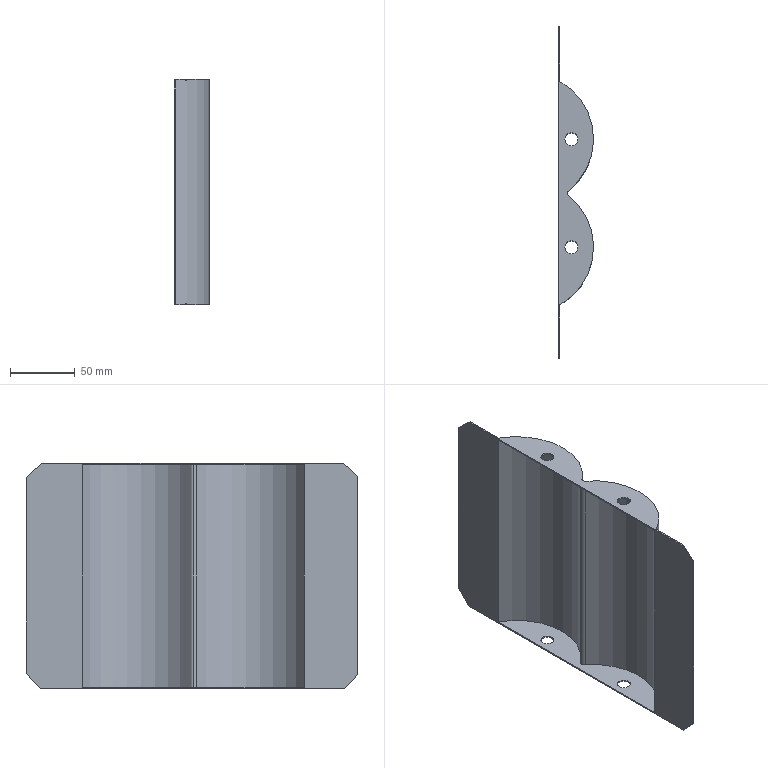Part | SolidWorks | features Chamfer 2, Extrusion 1, ICE 1, Shell 1 | 1 solid | 29 faces | box 27.127 x 256 x 174 mm | volume 56067 mm3 | cylinder 16 | plane 13 | commonest cylinder face diameters 10 x8 4 x2 6 x2 100 x2 102 x2
STEP:
#1=CARTESIAN_POINT('',(5.,168.7,173.));
#2=VERTEX_POINT('',#1);
#3=CARTESIAN_POINT('',(15.,168.7,173.));
#4=VERTEX_POINT('',#3);
#5=CARTESIAN_POINT('',(10.,168.7,173.));
#6=DIRECTION('',(0.,0.,1.));
#7=DIRECTION('',(1.,0.,0.));
#8=AXIS2_PLACEMENT_3D('',#5,#6,#7);
#9=CIRCLE('',#8,5.);
#10=EDGE_CURVE('',#2,#4,#9,.T.);
#11=ORIENTED_EDGE('',*,*,#10,.F.);
#12=CARTESIAN_POINT('',(5.,168.7,174.));
#13=VERTEX_POINT('',#12);
#14=CARTESIAN_POINT('',(5.,168.7,-28.));
#15=DIRECTION('',(0.,0.,1.));
#16=VECTOR('',#15,1000.);
#17=LINE('',#14,#16);
#18=EDGE_CURVE('',#2,#13,#17,.T.);
#19=ORIENTED_EDGE('',*,*,#18,.T.);
#20=CARTESIAN_POINT('',(15.,168.7,174.));
#21=VERTEX_POINT('',#20);
#22=CARTESIAN_POINT('',(10.,168.7,174.));
#23=DIRECTION('',(0.,0.,1.));
#24=DIRECTION('',(1.,0.,0.));
#25=AXIS2_PLACEMENT_3D('',#22,#23,#24);
#26=CIRCLE('',#25,5.);
#27=EDGE_CURVE('',#13,#21,#26,.T.);
#28=ORIENTED_EDGE('',*,*,#27,.T.);
#29=CARTESIAN_POINT('',(15.,168.7,-28.));
#30=DIRECTION('',(0.,0.,1.));
#31=VECTOR('',#30,1000.);
#32=LINE('',#29,#31);
#33=EDGE_CURVE('',#4,#21,#32,.T.);
#34=ORIENTED_EDGE('',*,*,#33,.F.);
#35=EDGE_LOOP('',(#11,#19,#28,#34));
#36=FACE_OUTER_BOUND('',#35,.T.);
#37=CARTESIAN_POINT('',(10.,168.7,-28.));
#38=DIRECTION('',(0.,0.,1.));
#39=DIRECTION('',(1.,0.,0.));
#40=AXIS2_PLACEMENT_3D('',#37,#38,#39);
#41=CYLINDRICAL_SURFACE('',#40,5.);
#42=ADVANCED_FACE('',(#36),#41,.F.);
#43=CARTESIAN_POINT('',(5.,85.3,173.));
#44=VERTEX_POINT('',#43);
#45=CARTESIAN_POINT('',(15.,85.3,173.));
#46=VERTEX_POINT('',#45);
#47=CARTESIAN_POINT('',(10.,85.3,173.));
#48=DIRECTION('',(0.,0.,1.));
#49=DIRECTION('',(1.,0.,0.));
#50=AXIS2_PLACEMENT_3D('',#47,#48,#49);
#51=CIRCLE('',#50,5.);
#52=EDGE_CURVE('',#44,#46,#51,.T.);
#53=ORIENTED_EDGE('',*,*,#52,.F.);
#54=CARTESIAN_POINT('',(5.,85.3,174.));
#55=VERTEX_POINT('',#54);
#56=CARTESIAN_POINT('',(5.,85.3,-28.));
#57=DIRECTION('',(0.,0.,1.));
#58=VECTOR('',#57,1000.);
#59=LINE('',#56,#58);
#60=EDGE_CURVE('',#44,#55,#59,.T.);
#61=ORIENTED_EDGE('',*,*,#60,.T.);
#62=CARTESIAN_POINT('',(15.,85.3,174.));
#63=VERTEX_POINT('',#62);
#64=CARTESIAN_POINT('',(10.,85.3,174.));
#65=DIRECTION('',(0.,0.,1.));
#66=DIRECTION('',(1.,0.,0.));
#67=AXIS2_PLACEMENT_3D('',#64,#65,#66);
#68=CIRCLE('',#67,5.);
#69=EDGE_CURVE('',#55,#63,#68,.T.);
#70=ORIENTED_EDGE('',*,*,#69,.T.);
#71=CARTESIAN_POINT('',(15.,85.3,-28.));
#72=DIRECTION('',(0.,0.,1.));
#73=VECTOR('',#72,1000.);
#74=LINE('',#71,#73);
#75=EDGE_CURVE('',#46,#63,#74,.T.);
#76=ORIENTED_EDGE('',*,*,#75,.F.);
#77=EDGE_LOOP('',(#53,#61,#70,#76));
#78=FACE_OUTER_BOUND('',#77,.T.);
#79=CARTESIAN_POINT('',(10.,85.3,-28.));
#80=DIRECTION('',(0.,0.,1.));
#81=DIRECTION('',(1.,0.,0.));
#82=AXIS2_PLACEMENT_3D('',#79,#80,#81);
#83=CYLINDRICAL_SURFACE('',#82,5.);
#84=ADVANCED_FACE('',(#78),#83,.F.);
#85=CARTESIAN_POINT('',(5.,168.7,0.));
#86=VERTEX_POINT('',#85);
#87=CARTESIAN_POINT('',(15.,168.7,0.));
#88=VERTEX_POINT('',#87);
#89=CARTESIAN_POINT('',(10.,168.7,0.));
#90=DIRECTION('',(0.,0.,1.));
#91=DIRECTION('',(1.,0.,0.));
#92=AXIS2_PLACEMENT_3D('',#89,#90,#91);
#93=CIRCLE('',#92,5.);
#94=EDGE_CURVE('',#86,#88,#93,.T.);
#95=ORIENTED_EDGE('',*,*,#94,.F.);
#96=CARTESIAN_POINT('',(5.,168.7,1.));
#97=VERTEX_POINT('',#96);
#98=CARTESIAN_POINT('',(5.,168.7,-28.));
#99=DIRECTION('',(0.,0.,1.));
#100=VECTOR('',#99,1000.);
#101=LINE('',#98,#100);
#102=EDGE_CURVE('',#86,#97,#101,.T.);
#103=ORIENTED_EDGE('',*,*,#102,.T.);
#104=CARTESIAN_POINT('',(15.,168.7,1.));
#105=VERTEX_POINT('',#104);
#106=CARTESIAN_POINT('',(10.,168.7,1.));
#107=DIRECTION('',(0.,0.,1.));
#108=DIRECTION('',(1.,0.,0.));
#109=AXIS2_PLACEMENT_3D('',#106,#107,#108);
#110=CIRCLE('',#109,5.);
#111=EDGE_CURVE('',#97,#105,#110,.T.);
#112=ORIENTED_EDGE('',*,*,#111,.T.);
#113=CARTESIAN_POINT('',(15.,168.7,-28.));
#114=DIRECTION('',(0.,0.,1.));
#115=VECTOR('',#114,1000.);
#116=LINE('',#113,#115);
#117=EDGE_CURVE('',#88,#105,#116,.T.);
#118=ORIENTED_EDGE('',*,*,#117,.F.);
#119=EDGE_LOOP('',(#95,#103,#112,#118));
#120=FACE_OUTER_BOUND('',#119,.T.);
#121=CARTESIAN_POINT('',(10.,168.7,-28.));
#122=DIRECTION('',(0.,0.,1.));
#123=DIRECTION('',(1.,0.,0.));
#124=AXIS2_PLACEMENT_3D('',#121,#122,#123);
#125=CYLINDRICAL_SURFACE('',#124,5.);
#126=ADVANCED_FACE('',(#120),#125,.F.);
#127=CARTESIAN_POINT('',(5.,85.3,0.));
#128=VERTEX_POINT('',#127);
#129=CARTESIAN_POINT('',(15.,85.3,0.));
#130=VERTEX_POINT('',#129);
#131=CARTESIAN_POINT('',(10.,85.3,0.));
#132=DIRECTION('',(0.,0.,1.));
#133=DIRECTION('',(1.,0.,0.));
#134=AXIS2_PLACEMENT_3D('',#131,#132,#133);
#135=CIRCLE('',#134,5.);
#136=EDGE_CURVE('',#128,#130,#135,.T.);
#137=ORIENTED_EDGE('',*,*,#136,.F.);
#138=CARTESIAN_POINT('',(5.,85.3,1.));
#139=VERTEX_POINT('',#138);
#140=CARTESIAN_POINT('',(5.,85.3,-28.));
#141=DIRECTION('',(0.,0.,1.));
#142=VECTOR('',#141,1000.);
#143=LINE('',#140,#142);
#144=EDGE_CURVE('',#128,#139,#143,.T.);
#145=ORIENTED_EDGE('',*,*,#144,.T.);
#146=CARTESIAN_POINT('',(15.,85.3,1.));
#147=VERTEX_POINT('',#146);
#148=CARTESIAN_POINT('',(10.,85.3,1.));
#149=DIRECTION('',(0.,0.,1.));
#150=DIRECTION('',(1.,0.,0.));
#151=AXIS2_PLACEMENT_3D('',#148,#149,#150);
#152=CIRCLE('',#151,5.);
#153=EDGE_CURVE('',#139,#147,#152,.T.);
#154=ORIENTED_EDGE('',*,*,#153,.T.);
#155=CARTESIAN_POINT('',(15.,85.3,-28.));
#156=DIRECTION('',(0.,0.,1.));
#157=VECTOR('',#156,1000.);
#158=LINE('',#155,#157);
#159=EDGE_CURVE('',#130,#147,#158,.T.);
#160=ORIENTED_EDGE('',*,*,#159,.F.);
#161=EDGE_LOOP('',(#137,#145,#154,#160));
#162=FACE_OUTER_BOUND('',#161,.T.);
#163=CARTESIAN_POINT('',(10.,85.3,-28.));
#164=DIRECTION('',(0.,0.,1.));
#165=DIRECTION('',(1.,0.,0.));
#166=AXIS2_PLACEMENT_3D('',#163,#164,#165);
#167=CYLINDRICAL_SURFACE('',#166,5.);
#168=ADVANCED_FACE('',(#162),#167,.F.);
#169=CARTESIAN_POINT('',(6.988,124.64,173.));
#170=VERTEX_POINT('',#169);
#171=CARTESIAN_POINT('',(5.839,127.,173.));
#172=VERTEX_POINT('',#171);
#173=CARTESIAN_POINT('',(8.839,127.,173.));
#174=DIRECTION('',(0.,0.,-1.));
#175=DIRECTION('',(1.,0.,0.));
#176=AXIS2_PLACEMENT_3D('',#173,#174,#175);
#177=CIRCLE('',#176,3.);
#178=EDGE_CURVE('',#170,#172,#177,.T.);
#179=ORIENTED_EDGE('',*,*,#178,.T.);
#180=CARTESIAN_POINT('',(5.839,127.,1.));
#181=VERTEX_POINT('',#180);
#182=CARTESIAN_POINT('',(5.839,127.,174.));
#183=DIRECTION('',(0.,0.,-1.));
#184=VECTOR('',#183,1000.);
#185=LINE('',#182,#184);
#186=EDGE_CURVE('',#172,#181,#185,.T.);
#187=ORIENTED_EDGE('',*,*,#186,.T.);
#188=CARTESIAN_POINT('',(6.988,124.64,1.));
#189=VERTEX_POINT('',#188);
#190=CARTESIAN_POINT('',(8.839,127.,1.));
#191=DIRECTION('',(0.,0.,-1.));
#192=DIRECTION('',(1.,0.,0.));
#193=AXIS2_PLACEMENT_3D('',#190,#191,#192);
#194=CIRCLE('',#193,3.);
#195=EDGE_CURVE('',#189,#181,#194,.T.);
#196=ORIENTED_EDGE('',*,*,#195,.F.);
#197=CARTESIAN_POINT('',(6.988,124.64,174.));
#198=DIRECTION('',(0.,0.,-1.));
#199=VECTOR('',#198,1000.);
#200=LINE('',#197,#199);
#201=EDGE_CURVE('',#170,#189,#200,.T.);
#202=ORIENTED_EDGE('',*,*,#201,.F.);
#203=EDGE_LOOP('',(#179,#187,#196,#202));
#204=FACE_OUTER_BOUND('',#203,.T.);
#205=CARTESIAN_POINT('',(8.839,127.,174.));
#206=DIRECTION('',(0.,0.,-1.));
#207=DIRECTION('',(-1.,0.,0.));
#208=AXIS2_PLACEMENT_3D('',#205,#206,#207);
#209=CYLINDRICAL_SURFACE('',#208,3.);
#210=ADVANCED_FACE('',(#204),#209,.T.);
#211=CARTESIAN_POINT('',(6.839,127.,174.));
#212=VERTEX_POINT('',#211);
#213=CARTESIAN_POINT('',(7.605,128.574,174.));
#214=VERTEX_POINT('',#213);
#215=CARTESIAN_POINT('',(8.839,127.,174.));
#216=DIRECTION('',(0.,0.,-1.));
#217=DIRECTION('',(1.,0.,0.));
#218=AXIS2_PLACEMENT_3D('',#215,#216,#217);
#219=CIRCLE('',#218,2.);
#220=EDGE_CURVE('',#212,#214,#219,.T.);
#221=ORIENTED_EDGE('',*,*,#220,.F.);
#222=CARTESIAN_POINT('',(6.839,127.,0.));
#223=VERTEX_POINT('',#222);
#224=CARTESIAN_POINT('',(6.839,127.,174.));
#225=DIRECTION('',(0.,0.,-1.));
#226=VECTOR('',#225,1000.);
#227=LINE('',#224,#226);
#228=EDGE_CURVE('',#212,#223,#227,.T.);
#229=ORIENTED_EDGE('',*,*,#228,.T.);
#230=CARTESIAN_POINT('',(7.605,128.574,0.));
#231=VERTEX_POINT('',#230);
#232=CARTESIAN_POINT('',(8.839,127.,0.));
#233=DIRECTION('',(0.,0.,-1.));
#234=DIRECTION('',(1.,0.,0.));
#235=AXIS2_PLACEMENT_3D('',#232,#233,#234);
#236=CIRCLE('',#235,2.);
#237=EDGE_CURVE('',#223,#231,#236,.T.);
#238=ORIENTED_EDGE('',*,*,#237,.T.);
#239=CARTESIAN_POINT('',(7.605,128.574,174.));
#240=DIRECTION('',(0.,0.,-1.));
#241=VECTOR('',#240,1000.);
#242=LINE('',#239,#241);
#243=EDGE_CURVE('',#214,#231,#242,.T.);
#244=ORIENTED_EDGE('',*,*,#243,.F.);
#245=EDGE_LOOP('',(#221,#229,#238,#244));
#246=FACE_OUTER_BOUND('',#245,.T.);
#247=CARTESIAN_POINT('',(8.839,127.,174.));
#248=DIRECTION('',(0.,0.,-1.));
#249=DIRECTION('',(-1.,0.,0.));
#250=AXIS2_PLACEMENT_3D('',#247,#248,#249);
#251=CYLINDRICAL_SURFACE('',#250,2.);
#252=ADVANCED_FACE('',(#246),#251,.F.);
#253=CARTESIAN_POINT('',(0.,11.,174.));
#254=VERTEX_POINT('',#253);
#255=CARTESIAN_POINT('',(0.,244.,174.));
#256=VERTEX_POINT('',#255);
#257=CARTESIAN_POINT('',(0.,0.,174.));
#258=DIRECTION('',(0.,1.,0.));
#259=VECTOR('',#258,1000.);
#260=LINE('',#257,#259);
#261=EDGE_CURVE('',#254,#256,#260,.T.);
#262=ORIENTED_EDGE('',*,*,#261,.T.);
#263=CARTESIAN_POINT('',(0.,256.,163.));
#264=VERTEX_POINT('',#263);
#265=CARTESIAN_POINT('',(0.,111.411,295.54));
#266=DIRECTION('',(0.,0.7372,-0.6757));
#267=VECTOR('',#266,1000.);
#268=LINE('',#265,#267);
#269=EDGE_CURVE('',#256,#264,#268,.T.);
#270=ORIENTED_EDGE('',*,*,#269,.T.);
#271=CARTESIAN_POINT('',(0.,256.,12.));
#272=VERTEX_POINT('',#271);
#273=CARTESIAN_POINT('',(0.,256.,174.));
#274=DIRECTION('',(0.,0.,-1.));
#275=VECTOR('',#274,1000.);
#276=LINE('',#273,#275);
#277=EDGE_CURVE('',#264,#272,#276,.T.);
#278=ORIENTED_EDGE('',*,*,#277,.T.);
#279=CARTESIAN_POINT('',(0.,245.,0.));
#280=VERTEX_POINT('',#279);
#281=CARTESIAN_POINT('',(0.,219.804,-27.487));
#282=DIRECTION('',(0.,-0.6757,-0.7372));
#283=VECTOR('',#282,1000.);
#284=LINE('',#281,#283);
#285=EDGE_CURVE('',#272,#280,#284,.T.);
#286=ORIENTED_EDGE('',*,*,#285,.T.);
#287=CARTESIAN_POINT('',(0.,10.,0.));
#288=VERTEX_POINT('',#287);
#289=CARTESIAN_POINT('',(0.,0.,0.));
#290=DIRECTION('',(0.,1.,0.));
#291=VECTOR('',#290,1000.);
#292=LINE('',#289,#291);
#293=EDGE_CURVE('',#288,#280,#292,.T.);
#294=ORIENTED_EDGE('',*,*,#293,.F.);
#295=CARTESIAN_POINT('',(0.,0.,11.));
#296=VERTEX_POINT('',#295);
#297=CARTESIAN_POINT('',(0.,-81.131,100.244));
#298=DIRECTION('',(0.,-0.6727,0.7399));
#299=VECTOR('',#298,1000.);
#300=LINE('',#297,#299);
#301=EDGE_CURVE('',#288,#296,#300,.T.);
#302=ORIENTED_EDGE('',*,*,#301,.T.);
#303=CARTESIAN_POINT('',(0.,0.,164.));
#304=VERTEX_POINT('',#303);
#305=CARTESIAN_POINT('',(0.,0.,174.));
#306=DIRECTION('',(0.,0.,-1.));
#307=VECTOR('',#306,1000.);
#308=LINE('',#305,#307);
#309=EDGE_CURVE('',#304,#296,#308,.T.);
#310=ORIENTED_EDGE('',*,*,#309,.F.);
#311=CARTESIAN_POINT('',(0.,4.977,168.525));
#312=DIRECTION('',(0.,0.7399,0.6727));
#313=VECTOR('',#312,1000.);
#314=LINE('',#311,#313);
#315=EDGE_CURVE('',#304,#254,#314,.T.);
#316=ORIENTED_EDGE('',*,*,#315,.T.);
#317=EDGE_LOOP('',(#262,#270,#278,#286,#294,#302,#310,#316));
#318=FACE_OUTER_BOUND('',#317,.T.);
#319=CARTESIAN_POINT('',(0.,41.367,173.));
#320=VERTEX_POINT('',#319);
#321=CARTESIAN_POINT('',(0.,212.633,173.));
#322=VERTEX_POINT('',#321);
#323=CARTESIAN_POINT('',(0.,0.,173.));
#324=DIRECTION('',(0.,1.,0.));
#325=VECTOR('',#324,1000.);
#326=LINE('',#323,#325);
#327=EDGE_CURVE('',#320,#322,#326,.T.);
#328=ORIENTED_EDGE('',*,*,#327,.F.);
#329=CARTESIAN_POINT('',(0.,41.367,1.));
#330=VERTEX_POINT('',#329);
#331=CARTESIAN_POINT('',(0.,41.367,173.));
#332=DIRECTION('',(0.,0.,-1.));
#333=VECTOR('',#332,1000.);
#334=LINE('',#331,#333);
#335=EDGE_CURVE('',#320,#330,#334,.T.);
#336=ORIENTED_EDGE('',*,*,#335,.T.);
#337=CARTESIAN_POINT('',(0.,212.633,1.));
#338=VERTEX_POINT('',#337);
#339=CARTESIAN_POINT('',(0.,0.,1.));
#340=DIRECTION('',(0.,1.,0.));
#341=VECTOR('',#340,1000.);
#342=LINE('',#339,#341);
#343=EDGE_CURVE('',#330,#338,#342,.T.);
#344=ORIENTED_EDGE('',*,*,#343,.T.);
#345=CARTESIAN_POINT('',(0.,212.633,173.));
#346=DIRECTION('',(0.,0.,-1.));
#347=VECTOR('',#346,1000.);
#348=LINE('',#345,#347);
#349=EDGE_CURVE('',#322,#338,#348,.T.);
#350=ORIENTED_EDGE('',*,*,#349,.F.);
#351=EDGE_LOOP('',(#328,#336,#344,#350));
#352=FACE_BOUND('',#351,.T.);
#353=CARTESIAN_POINT('',(0.,0.,174.));
#354=DIRECTION('',(-1.,0.,0.));
#355=DIRECTION('',(0.,-1.,0.));
#356=AXIS2_PLACEMENT_3D('',#353,#354,#355);
#357=PLANE('',#356);
#358=ADVANCED_FACE('',(#318,#352),#357,.T.);
#359=ORIENTED_EDGE('',*,*,#277,.F.);
#360=CARTESIAN_POINT('',(1.,256.,163.));
#361=VERTEX_POINT('',#360);
#362=CARTESIAN_POINT('',(0.,256.,163.));
#363=DIRECTION('',(1.,0.,0.));
#364=VECTOR('',#363,1000.);
#365=LINE('',#362,#364);
#366=EDGE_CURVE('',#264,#361,#365,.T.);
#367=ORIENTED_EDGE('',*,*,#366,.T.);
#368=CARTESIAN_POINT('',(1.,256.,12.));
#369=VERTEX_POINT('',#368);
#370=CARTESIAN_POINT('',(1.,256.,174.));
#371=DIRECTION('',(0.,0.,-1.));
#372=VECTOR('',#371,1000.);
#373=LINE('',#370,#372);
#374=EDGE_CURVE('',#361,#369,#373,.T.);
#375=ORIENTED_EDGE('',*,*,#374,.T.);
#376=CARTESIAN_POINT('',(0.,256.,12.));
#377=DIRECTION('',(-1.,0.,0.));
#378=VECTOR('',#377,1000.);
#379=LINE('',#376,#378);
#380=EDGE_CURVE('',#369,#272,#379,.T.);
#381=ORIENTED_EDGE('',*,*,#380,.T.);
#382=EDGE_LOOP('',(#359,#367,#375,#381));
#383=FACE_OUTER_BOUND('',#382,.T.);
#384=CARTESIAN_POINT('',(0.,256.,174.));
#385=DIRECTION('',(0.,1.,0.));
#386=DIRECTION('',(0.,0.,1.));
#387=AXIS2_PLACEMENT_3D('',#384,#385,#386);
#388=PLANE('',#387);
#389=ADVANCED_FACE('',(#383),#388,.T.);
#390=ORIENTED_EDGE('',*,*,#309,.T.);
#391=CARTESIAN_POINT('',(1.,0.,11.));
#392=VERTEX_POINT('',#391);
#393=CARTESIAN_POINT('',(0.,0.,11.));
#394=DIRECTION('',(1.,0.,0.));
#395=VECTOR('',#394,1000.);
#396=LINE('',#393,#395);
#397=EDGE_CURVE('',#296,#392,#396,.T.);
#398=ORIENTED_EDGE('',*,*,#397,.T.);
#399=CARTESIAN_POINT('',(1.,0.,164.));
#400=VERTEX_POINT('',#399);
#401=CARTESIAN_POINT('',(1.,0.,174.));
#402=DIRECTION('',(0.,0.,-1.));
#403=VECTOR('',#402,1000.);
#404=LINE('',#401,#403);
#405=EDGE_CURVE('',#400,#392,#404,.T.);
#406=ORIENTED_EDGE('',*,*,#405,.F.);
#407=CARTESIAN_POINT('',(0.,0.,164.));
#408=DIRECTION('',(-1.,0.,0.));
#409=VECTOR('',#408,1000.);
#410=LINE('',#407,#409);
#411=EDGE_CURVE('',#400,#304,#410,.T.);
#412=ORIENTED_EDGE('',*,*,#411,.T.);
#413=EDGE_LOOP('',(#390,#398,#406,#412));
#414=FACE_OUTER_BOUND('',#413,.T.);
#415=CARTESIAN_POINT('',(0.,0.,174.));
#416=DIRECTION('',(0.,1.,0.));
#417=DIRECTION('',(0.,0.,1.));
#418=AXIS2_PLACEMENT_3D('',#415,#416,#417);
#419=PLANE('',#418);
#420=ADVANCED_FACE('',(#414),#419,.F.);
#421=ORIENTED_EDGE('',*,*,#405,.T.);
#422=CARTESIAN_POINT('',(1.,10.,0.));
#423=VERTEX_POINT('',#422);
#424=CARTESIAN_POINT('',(1.,0.,11.));
#425=DIRECTION('',(0.,0.6727,-0.7399));
#426=VECTOR('',#425,1000.);
#427=LINE('',#424,#426);
#428=EDGE_CURVE('',#392,#423,#427,.T.);
#429=ORIENTED_EDGE('',*,*,#428,.T.);
#430=CARTESIAN_POINT('',(1.,40.777,0.));
#431=VERTEX_POINT('',#430);
#432=CARTESIAN_POINT('',(1.,0.,0.));
#433=DIRECTION('',(0.,1.,0.));
#434=VECTOR('',#433,1000.);
#435=LINE('',#432,#434);
#436=EDGE_CURVE('',#423,#431,#435,.T.);
#437=ORIENTED_EDGE('',*,*,#436,.T.);
#438=CARTESIAN_POINT('',(1.,40.777,174.));
#439=VERTEX_POINT('',#438);
#440=CARTESIAN_POINT('',(1.,40.777,174.));
#441=DIRECTION('',(0.,0.,-1.));
#442=VECTOR('',#441,1000.);
#443=LINE('',#440,#442);
#444=EDGE_CURVE('',#439,#431,#443,.T.);
#445=ORIENTED_EDGE('',*,*,#444,.F.);
#446=CARTESIAN_POINT('',(1.,11.,174.));
#447=VERTEX_POINT('',#446);
#448=CARTESIAN_POINT('',(1.,0.,174.));
#449=DIRECTION('',(0.,1.,0.));
#450=VECTOR('',#449,1000.);
#451=LINE('',#448,#450);
#452=EDGE_CURVE('',#447,#439,#451,.T.);
#453=ORIENTED_EDGE('',*,*,#452,.F.);
#454=CARTESIAN_POINT('',(1.,11.,174.));
#455=DIRECTION('',(0.,-0.7399,-0.6727));
#456=VECTOR('',#455,1000.);
#457=LINE('',#454,#456);
#458=EDGE_CURVE('',#447,#400,#457,.T.);
#459=ORIENTED_EDGE('',*,*,#458,.T.);
#460=EDGE_LOOP('',(#421,#429,#437,#445,#453,#459));
#461=FACE_OUTER_BOUND('',#460,.T.);
#462=CARTESIAN_POINT('',(1.,0.,174.));
#463=DIRECTION('',(-1.,0.,0.));
#464=DIRECTION('',(0.,-1.,0.));
#465=AXIS2_PLACEMENT_3D('',#462,#463,#464);
#466=PLANE('',#465);
#467=ADVANCED_FACE('',(#461),#466,.F.);
#468=CARTESIAN_POINT('',(7.605,125.426,0.));
#469=VERTEX_POINT('',#468);
#470=CARTESIAN_POINT('',(-23.873,85.3,0.));
#471=DIRECTION('',(0.,0.,-1.));
#472=DIRECTION('',(1.,0.,0.));
#473=AXIS2_PLACEMENT_3D('',#470,#471,#472);
#474=CIRCLE('',#473,51.);
#475=EDGE_CURVE('',#469,#431,#474,.T.);
#476=ORIENTED_EDGE('',*,*,#475,.F.);
#477=CARTESIAN_POINT('',(7.605,125.426,174.));
#478=VERTEX_POINT('',#477);
#479=CARTESIAN_POINT('',(7.605,125.426,174.));
#480=DIRECTION('',(0.,0.,-1.));
#481=VECTOR('',#480,1000.);
#482=LINE('',#479,#481);
#483=EDGE_CURVE('',#478,#469,#482,.T.);
#484=ORIENTED_EDGE('',*,*,#483,.F.);
#485=CARTESIAN_POINT('',(-23.873,85.3,174.));
#486=DIRECTION('',(0.,0.,-1.));
#487=DIRECTION('',(1.,0.,0.));
#488=AXIS2_PLACEMENT_3D('',#485,#486,#487);
#489=CIRCLE('',#488,51.);
#490=EDGE_CURVE('',#478,#439,#489,.T.);
#491=ORIENTED_EDGE('',*,*,#490,.T.);
#492=ORIENTED_EDGE('',*,*,#444,.T.);
#493=EDGE_LOOP('',(#476,#484,#491,#492));
#494=FACE_OUTER_BOUND('',#493,.T.);
#495=CARTESIAN_POINT('',(-23.873,85.3,174.));
#496=DIRECTION('',(0.,0.,-1.));
#497=DIRECTION('',(-1.,0.,0.));
#498=AXIS2_PLACEMENT_3D('',#495,#496,#497);
#499=CYLINDRICAL_SURFACE('',#498,51.);
#500=ADVANCED_FACE('',(#494),#499,.T.);
#501=ORIENTED_EDGE('',*,*,#228,.F.);
#502=CARTESIAN_POINT('',(8.839,127.,174.));
#503=DIRECTION('',(0.,0.,-1.));
#504=DIRECTION('',(1.,0.,0.));
#505=AXIS2_PLACEMENT_3D('',#502,#503,#504);
#506=CIRCLE('',#505,2.);
#507=EDGE_CURVE('',#478,#212,#506,.T.);
#508=ORIENTED_EDGE('',*,*,#507,.F.);
#509=ORIENTED_EDGE('',*,*,#483,.T.);
#510=CARTESIAN_POINT('',(8.839,127.,0.));
#511=DIRECTION('',(0.,0.,-1.));
#512=DIRECTION('',(1.,0.,0.));
#513=AXIS2_PLACEMENT_3D('',#510,#511,#512);
#514=CIRCLE('',#513,2.);
#515=EDGE_CURVE('',#469,#223,#514,.T.);
#516=ORIENTED_EDGE('',*,*,#515,.T.);
#517=EDGE_LOOP('',(#501,#508,#509,#516));
#518=FACE_OUTER_BOUND('',#517,.T.);
#519=CARTESIAN_POINT('',(8.839,127.,174.));
#520=DIRECTION('',(0.,0.,-1.));
#521=DIRECTION('',(-1.,0.,0.));
#522=AXIS2_PLACEMENT_3D('',#519,#520,#521);
#523=CYLINDRICAL_SURFACE('',#522,2.);
#524=ADVANCED_FACE('',(#518),#523,.F.);
#525=CARTESIAN_POINT('',(1.,213.223,0.));
#526=VERTEX_POINT('',#525);
#527=CARTESIAN_POINT('',(-23.873,168.7,0.));
#528=DIRECTION('',(0.,0.,-1.));
#529=DIRECTION('',(1.,0.,0.));
#530=AXIS2_PLACEMENT_3D('',#527,#528,#529);
#531=CIRCLE('',#530,51.);
#532=EDGE_CURVE('',#526,#231,#531,.T.);
#533=ORIENTED_EDGE('',*,*,#532,.F.);
#534=CARTESIAN_POINT('',(1.,213.223,174.));
#535=VERTEX_POINT('',#534);
#536=CARTESIAN_POINT('',(1.,213.223,174.));
#537=DIRECTION('',(0.,0.,-1.));
#538=VECTOR('',#537,1000.);
#539=LINE('',#536,#538);
#540=EDGE_CURVE('',#535,#526,#539,.T.);
#541=ORIENTED_EDGE('',*,*,#540,.F.);
#542=CARTESIAN_POINT('',(-23.873,168.7,174.));
#543=DIRECTION('',(0.,0.,-1.));
#544=DIRECTION('',(1.,0.,0.));
#545=AXIS2_PLACEMENT_3D('',#542,#543,#544);
#546=CIRCLE('',#545,51.);
#547=EDGE_CURVE('',#535,#214,#546,.T.);
#548=ORIENTED_EDGE('',*,*,#547,.T.);
#549=ORIENTED_EDGE('',*,*,#243,.T.);
#550=EDGE_LOOP('',(#533,#541,#548,#549));
#551=FACE_OUTER_BOUND('',#550,.T.);
#552=CARTESIAN_POINT('',(-23.873,168.7,174.));
#553=DIRECTION('',(0.,0.,-1.));
#554=DIRECTION('',(-1.,0.,0.));
#555=AXIS2_PLACEMENT_3D('',#552,#553,#554);
#556=CYLINDRICAL_SURFACE('',#555,51.);
#557=ADVANCED_FACE('',(#551),#556,.T.);
#558=ORIENTED_EDGE('',*,*,#374,.F.);
#559=CARTESIAN_POINT('',(1.,244.,174.));
#560=VERTEX_POINT('',#559);
#561=CARTESIAN_POINT('',(1.,256.,163.));
#562=DIRECTION('',(0.,-0.7372,0.6757));
#563=VECTOR('',#562,1000.);
#564=LINE('',#561,#563);
#565=EDGE_CURVE('',#361,#560,#564,.T.);
#566=ORIENTED_EDGE('',*,*,#565,.T.);
#567=CARTESIAN_POINT('',(1.,0.,174.));
#568=DIRECTION('',(0.,1.,0.));
#569=VECTOR('',#568,1000.);
#570=LINE('',#567,#569);
#571=EDGE_CURVE('',#535,#560,#570,.T.);
#572=ORIENTED_EDGE('',*,*,#571,.F.);
#573=ORIENTED_EDGE('',*,*,#540,.T.);
#574=CARTESIAN_POINT('',(1.,245.,0.));
#575=VERTEX_POINT('',#574);
#576=CARTESIAN_POINT('',(1.,0.,0.));
#577=DIRECTION('',(0.,1.,0.));
#578=VECTOR('',#577,1000.);
#579=LINE('',#576,#578);
#580=EDGE_CURVE('',#526,#575,#579,.T.);
#581=ORIENTED_EDGE('',*,*,#580,.T.);
#582=CARTESIAN_POINT('',(1.,245.,0.));
#583=DIRECTION('',(0.,0.6757,0.7372));
#584=VECTOR('',#583,1000.);
#585=LINE('',#582,#584);
#586=EDGE_CURVE('',#575,#369,#585,.T.);
#587=ORIENTED_EDGE('',*,*,#586,.T.);
#588=EDGE_LOOP('',(#558,#566,#572,#573,#581,#587));
#589=FACE_OUTER_BOUND('',#588,.T.);
#590=CARTESIAN_POINT('',(1.,0.,174.));
#591=DIRECTION('',(-1.,0.,0.));
#592=DIRECTION('',(0.,-1.,0.));
#593=AXIS2_PLACEMENT_3D('',#590,#591,#592);
#594=PLANE('',#593);
#595=ADVANCED_FACE('',(#589),#594,.F.);
#596=CARTESIAN_POINT('',(10.,168.7,174.));
#597=DIRECTION('',(0.,0.,1.));
#598=DIRECTION('',(1.,0.,0.));
#599=AXIS2_PLACEMENT_3D('',#596,#597,#598);
#600=CIRCLE('',#599,5.);
#601=EDGE_CURVE('',#21,#13,#600,.T.);
#602=ORIENTED_EDGE('',*,*,#601,.F.);
#603=ORIENTED_EDGE('',*,*,#27,.F.);
#604=EDGE_LOOP('',(#602,#603));
#605=FACE_BOUND('',#604,.T.);
#606=CARTESIAN_POINT('',(10.,85.3,174.));
#607=DIRECTION('',(0.,0.,1.));
#608=DIRECTION('',(1.,0.,0.));
#609=AXIS2_PLACEMENT_3D('',#606,#607,#608);
#610=CIRCLE('',#609,5.);
#611=EDGE_CURVE('',#63,#55,#610,.T.);
#612=ORIENTED_EDGE('',*,*,#611,.F.);
#613=ORIENTED_EDGE('',*,*,#69,.F.);
#614=EDGE_LOOP('',(#612,#613));
#615=FACE_BOUND('',#614,.T.);
#616=ORIENTED_EDGE('',*,*,#571,.T.);
#617=CARTESIAN_POINT('',(0.,244.,174.));
#618=DIRECTION('',(-1.,0.,0.));
#619=VECTOR('',#618,1000.);
#620=LINE('',#617,#619);
#621=EDGE_CURVE('',#560,#256,#620,.T.);
#622=ORIENTED_EDGE('',*,*,#621,.T.);
#623=ORIENTED_EDGE('',*,*,#261,.F.);
#624=CARTESIAN_POINT('',(1.,11.,174.));
#625=DIRECTION('',(1.,0.,0.));
#626=VECTOR('',#625,1000.);
#627=LINE('',#624,#626);
#628=EDGE_CURVE('',#254,#447,#627,.T.);
#629=ORIENTED_EDGE('',*,*,#628,.T.);
#630=ORIENTED_EDGE('',*,*,#452,.T.);
#631=ORIENTED_EDGE('',*,*,#490,.F.);
#632=ORIENTED_EDGE('',*,*,#507,.T.);
#633=ORIENTED_EDGE('',*,*,#220,.T.);
#634=ORIENTED_EDGE('',*,*,#547,.F.);
#635=EDGE_LOOP('',(#616,#622,#623,#629,#630,#631,#632,#633,#634));
#636=FACE_OUTER_BOUND('',#635,.T.);
#637=CARTESIAN_POINT('',(0.,0.,174.));
#638=DIRECTION('',(0.,0.,1.));
#639=DIRECTION('',(1.,0.,0.));
#640=AXIS2_PLACEMENT_3D('',#637,#638,#639);
#641=PLANE('',#640);
#642=ADVANCED_FACE('',(#605,#615,#636),#641,.T.);
#643=CARTESIAN_POINT('',(10.,168.7,0.));
#644=DIRECTION('',(0.,0.,1.));
#645=DIRECTION('',(1.,0.,0.));
#646=AXIS2_PLACEMENT_3D('',#643,#644,#645);
#647=CIRCLE('',#646,5.);
#648=EDGE_CURVE('',#88,#86,#647,.T.);
#649=ORIENTED_EDGE('',*,*,#648,.T.);
#650=ORIENTED_EDGE('',*,*,#94,.T.);
#651=EDGE_LOOP('',(#649,#650));
#652=FACE_BOUND('',#651,.T.);
#653=CARTESIAN_POINT('',(10.,85.3,0.));
#654=DIRECTION('',(0.,0.,1.));
#655=DIRECTION('',(1.,0.,0.));
#656=AXIS2_PLACEMENT_3D('',#653,#654,#655);
#657=CIRCLE('',#656,5.);
#658=EDGE_CURVE('',#130,#128,#657,.T.);
#659=ORIENTED_EDGE('',*,*,#658,.T.);
#660=ORIENTED_EDGE('',*,*,#136,.T.);
#661=EDGE_LOOP('',(#659,#660));
#662=FACE_BOUND('',#661,.T.);
#663=ORIENTED_EDGE('',*,*,#293,.T.);
#664=CARTESIAN_POINT('',(1.,245.,0.));
#665=DIRECTION('',(1.,0.,0.));
#666=VECTOR('',#665,1000.);
#667=LINE('',#664,#666);
#668=EDGE_CURVE('',#280,#575,#667,.T.);
#669=ORIENTED_EDGE('',*,*,#668,.T.);
#670=ORIENTED_EDGE('',*,*,#580,.F.);
#671=ORIENTED_EDGE('',*,*,#532,.T.);
#672=ORIENTED_EDGE('',*,*,#237,.F.);
#673=ORIENTED_EDGE('',*,*,#515,.F.);
#674=ORIENTED_EDGE('',*,*,#475,.T.);
#675=ORIENTED_EDGE('',*,*,#436,.F.);
#676=CARTESIAN_POINT('',(0.,10.,0.));
#677=DIRECTION('',(-1.,0.,0.));
#678=VECTOR('',#677,1000.);
#679=LINE('',#676,#678);
#680=EDGE_CURVE('',#423,#288,#679,.T.);
#681=ORIENTED_EDGE('',*,*,#680,.T.);
#682=EDGE_LOOP('',(#663,#669,#670,#671,#672,#673,#674,#675,#681));
#683=FACE_OUTER_BOUND('',#682,.T.);
#684=CARTESIAN_POINT('',(0.,0.,0.));
#685=DIRECTION('',(0.,0.,1.));
#686=DIRECTION('',(1.,0.,0.));
#687=AXIS2_PLACEMENT_3D('',#684,#685,#686);
#688=PLANE('',#687);
#689=ADVANCED_FACE('',(#652,#662,#683),#688,.F.);
#690=CARTESIAN_POINT('',(-23.873,85.3,1.));
#691=DIRECTION('',(0.,0.,-1.));
#692=DIRECTION('',(1.,0.,0.));
#693=AXIS2_PLACEMENT_3D('',#690,#691,#692);
#694=CIRCLE('',#693,50.);
#695=EDGE_CURVE('',#189,#330,#694,.T.);
#696=ORIENTED_EDGE('',*,*,#695,.T.);
#697=ORIENTED_EDGE('',*,*,#335,.F.);
#698=CARTESIAN_POINT('',(-23.873,85.3,173.));
#699=DIRECTION('',(0.,0.,-1.));
#700=DIRECTION('',(1.,0.,0.));
#701=AXIS2_PLACEMENT_3D('',#698,#699,#700);
#702=CIRCLE('',#701,50.);
#703=EDGE_CURVE('',#170,#320,#702,.T.);
#704=ORIENTED_EDGE('',*,*,#703,.F.);
#705=ORIENTED_EDGE('',*,*,#201,.T.);
#706=EDGE_LOOP('',(#696,#697,#704,#705));
#707=FACE_OUTER_BOUND('',#706,.T.);
#708=CARTESIAN_POINT('',(-23.873,85.3,174.));
#709=DIRECTION('',(0.,0.,-1.));
#710=DIRECTION('',(-1.,0.,0.));
#711=AXIS2_PLACEMENT_3D('',#708,#709,#710);
#712=CYLINDRICAL_SURFACE('',#711,50.);
#713=ADVANCED_FACE('',(#707),#712,.F.);
#714=ORIENTED_EDGE('',*,*,#186,.F.);
#715=CARTESIAN_POINT('',(6.988,129.36,173.));
#716=VERTEX_POINT('',#715);
#717=CARTESIAN_POINT('',(8.839,127.,173.));
#718=DIRECTION('',(0.,0.,-1.));
#719=DIRECTION('',(1.,0.,0.));
#720=AXIS2_PLACEMENT_3D('',#717,#718,#719);
#721=CIRCLE('',#720,3.);
#722=EDGE_CURVE('',#172,#716,#721,.T.);
#723=ORIENTED_EDGE('',*,*,#722,.T.);
#724=CARTESIAN_POINT('',(6.988,129.36,1.));
#725=VERTEX_POINT('',#724);
#726=CARTESIAN_POINT('',(6.988,129.36,174.));
#727=DIRECTION('',(0.,0.,-1.));
#728=VECTOR('',#727,1000.);
#729=LINE('',#726,#728);
#730=EDGE_CURVE('',#716,#725,#729,.T.);
#731=ORIENTED_EDGE('',*,*,#730,.T.);
#732=CARTESIAN_POINT('',(8.839,127.,1.));
#733=DIRECTION('',(0.,0.,-1.));
#734=DIRECTION('',(1.,0.,0.));
#735=AXIS2_PLACEMENT_3D('',#732,#733,#734);
#736=CIRCLE('',#735,3.);
#737=EDGE_CURVE('',#181,#725,#736,.T.);
#738=ORIENTED_EDGE('',*,*,#737,.F.);
#739=EDGE_LOOP('',(#714,#723,#731,#738));
#740=FACE_OUTER_BOUND('',#739,.T.);
#741=CARTESIAN_POINT('',(8.839,127.,174.));
#742=DIRECTION('',(0.,0.,-1.));
#743=DIRECTION('',(-1.,0.,0.));
#744=AXIS2_PLACEMENT_3D('',#741,#742,#743);
#745=CYLINDRICAL_SURFACE('',#744,3.);
#746=ADVANCED_FACE('',(#740),#745,.T.);
#747=CARTESIAN_POINT('',(-23.873,168.7,1.));
#748=DIRECTION('',(0.,0.,-1.));
#749=DIRECTION('',(1.,0.,0.));
#750=AXIS2_PLACEMENT_3D('',#747,#748,#749);
#751=CIRCLE('',#750,50.);
#752=EDGE_CURVE('',#338,#725,#751,.T.);
#753=ORIENTED_EDGE('',*,*,#752,.T.);
#754=ORIENTED_EDGE('',*,*,#730,.F.);
#755=CARTESIAN_POINT('',(-23.873,168.7,173.));
#756=DIRECTION('',(0.,0.,-1.));
#757=DIRECTION('',(1.,0.,0.));
#758=AXIS2_PLACEMENT_3D('',#755,#756,#757);
#759=CIRCLE('',#758,50.);
#760=EDGE_CURVE('',#322,#716,#759,.T.);
#761=ORIENTED_EDGE('',*,*,#760,.F.);
#762=ORIENTED_EDGE('',*,*,#349,.T.);
#763=EDGE_LOOP('',(#753,#754,#761,#762));
#764=FACE_OUTER_BOUND('',#763,.T.);
#765=CARTESIAN_POINT('',(-23.873,168.7,174.));
#766=DIRECTION('',(0.,0.,-1.));
#767=DIRECTION('',(-1.,0.,0.));
#768=AXIS2_PLACEMENT_3D('',#765,#766,#767);
#769=CYLINDRICAL_SURFACE('',#768,50.);
#770=ADVANCED_FACE('',(#764),#769,.F.);
#771=CARTESIAN_POINT('',(10.,168.7,173.));
#772=DIRECTION('',(0.,0.,1.));
#773=DIRECTION('',(1.,0.,0.));
#774=AXIS2_PLACEMENT_3D('',#771,#772,#773);
#775=CIRCLE('',#774,5.);
#776=EDGE_CURVE('',#4,#2,#775,.T.);
#777=ORIENTED_EDGE('',*,*,#776,.T.);
#778=ORIENTED_EDGE('',*,*,#10,.T.);
#779=EDGE_LOOP('',(#777,#778));
#780=FACE_BOUND('',#779,.T.);
#781=CARTESIAN_POINT('',(10.,85.3,173.));
#782=DIRECTION('',(0.,0.,1.));
#783=DIRECTION('',(1.,0.,0.));
#784=AXIS2_PLACEMENT_3D('',#781,#782,#783);
#785=CIRCLE('',#784,5.);
#786=EDGE_CURVE('',#46,#44,#785,.T.);
#787=ORIENTED_EDGE('',*,*,#786,.T.);
#788=ORIENTED_EDGE('',*,*,#52,.T.);
#789=EDGE_LOOP('',(#787,#788));
#790=FACE_BOUND('',#789,.T.);
#791=ORIENTED_EDGE('',*,*,#760,.T.);
#792=ORIENTED_EDGE('',*,*,#722,.F.);
#793=ORIENTED_EDGE('',*,*,#178,.F.);
#794=ORIENTED_EDGE('',*,*,#703,.T.);
#795=ORIENTED_EDGE('',*,*,#327,.T.);
#796=EDGE_LOOP('',(#791,#792,#793,#794,#795));
#797=FACE_OUTER_BOUND('',#796,.T.);
#798=CARTESIAN_POINT('',(0.,0.,173.));
#799=DIRECTION('',(0.,0.,1.));
#800=DIRECTION('',(1.,0.,0.));
#801=AXIS2_PLACEMENT_3D('',#798,#799,#800);
#802=PLANE('',#801);
#803=ADVANCED_FACE('',(#780,#790,#797),#802,.F.);
#804=CARTESIAN_POINT('',(10.,168.7,1.));
#805=DIRECTION('',(0.,0.,1.));
#806=DIRECTION('',(1.,0.,0.));
#807=AXIS2_PLACEMENT_3D('',#804,#805,#806);
#808=CIRCLE('',#807,5.);
#809=EDGE_CURVE('',#105,#97,#808,.T.);
#810=ORIENTED_EDGE('',*,*,#809,.F.);
#811=ORIENTED_EDGE('',*,*,#111,.F.);
#812=EDGE_LOOP('',(#810,#811));
#813=FACE_BOUND('',#812,.T.);
#814=CARTESIAN_POINT('',(10.,85.3,1.));
#815=DIRECTION('',(0.,0.,1.));
#816=DIRECTION('',(1.,0.,0.));
#817=AXIS2_PLACEMENT_3D('',#814,#815,#816);
#818=CIRCLE('',#817,5.);
#819=EDGE_CURVE('',#147,#139,#818,.T.);
#820=ORIENTED_EDGE('',*,*,#819,.F.);
#821=ORIENTED_EDGE('',*,*,#153,.F.);
#822=EDGE_LOOP('',(#820,#821));
#823=FACE_BOUND('',#822,.T.);
#824=ORIENTED_EDGE('',*,*,#695,.F.);
#825=ORIENTED_EDGE('',*,*,#195,.T.);
#826=ORIENTED_EDGE('',*,*,#737,.T.);
#827=ORIENTED_EDGE('',*,*,#752,.F.);
#828=ORIENTED_EDGE('',*,*,#343,.F.);
#829=EDGE_LOOP('',(#824,#825,#826,#827,#828));
#830=FACE_OUTER_BOUND('',#829,.T.);
#831=CARTESIAN_POINT('',(0.,0.,1.));
#832=DIRECTION('',(0.,0.,1.));
#833=DIRECTION('',(1.,0.,0.));
#834=AXIS2_PLACEMENT_3D('',#831,#832,#833);
#835=PLANE('',#834);
#836=ADVANCED_FACE('',(#813,#823,#830),#835,.T.);
#837=ORIENTED_EDGE('',*,*,#144,.F.);
#838=ORIENTED_EDGE('',*,*,#658,.F.);
#839=ORIENTED_EDGE('',*,*,#159,.T.);
#840=ORIENTED_EDGE('',*,*,#819,.T.);
#841=EDGE_LOOP('',(#837,#838,#839,#840));
#842=FACE_OUTER_BOUND('',#841,.T.);
#843=CARTESIAN_POINT('',(10.,85.3,-28.));
#844=DIRECTION('',(0.,0.,1.));
#845=DIRECTION('',(1.,0.,0.));
#846=AXIS2_PLACEMENT_3D('',#843,#844,#845);
#847=CYLINDRICAL_SURFACE('',#846,5.);
#848=ADVANCED_FACE('',(#842),#847,.F.);
#849=ORIENTED_EDGE('',*,*,#102,.F.);
#850=ORIENTED_EDGE('',*,*,#648,.F.);
#851=ORIENTED_EDGE('',*,*,#117,.T.);
#852=ORIENTED_EDGE('',*,*,#809,.T.);
#853=EDGE_LOOP('',(#849,#850,#851,#852));
#854=FACE_OUTER_BOUND('',#853,.T.);
#855=CARTESIAN_POINT('',(10.,168.7,-28.));
#856=DIRECTION('',(0.,0.,1.));
#857=DIRECTION('',(1.,0.,0.));
#858=AXIS2_PLACEMENT_3D('',#855,#856,#857);
#859=CYLINDRICAL_SURFACE('',#858,5.);
#860=ADVANCED_FACE('',(#854),#859,.F.);
#861=ORIENTED_EDGE('',*,*,#60,.F.);
#862=ORIENTED_EDGE('',*,*,#786,.F.);
#863=ORIENTED_EDGE('',*,*,#75,.T.);
#864=ORIENTED_EDGE('',*,*,#611,.T.);
#865=EDGE_LOOP('',(#861,#862,#863,#864));
#866=FACE_OUTER_BOUND('',#865,.T.);
#867=CARTESIAN_POINT('',(10.,85.3,-28.));
#868=DIRECTION('',(0.,0.,1.));
#869=DIRECTION('',(1.,0.,0.));
#870=AXIS2_PLACEMENT_3D('',#867,#868,#869);
#871=CYLINDRICAL_SURFACE('',#870,5.);
#872=ADVANCED_FACE('',(#866),#871,.F.);
#873=ORIENTED_EDGE('',*,*,#18,.F.);
#874=ORIENTED_EDGE('',*,*,#776,.F.);
#875=ORIENTED_EDGE('',*,*,#33,.T.);
#876=ORIENTED_EDGE('',*,*,#601,.T.);
#877=EDGE_LOOP('',(#873,#874,#875,#876));
#878=FACE_OUTER_BOUND('',#877,.T.);
#879=CARTESIAN_POINT('',(10.,168.7,-28.));
#880=DIRECTION('',(0.,0.,1.));
#881=DIRECTION('',(1.,0.,0.));
#882=AXIS2_PLACEMENT_3D('',#879,#880,#881);
#883=CYLINDRICAL_SURFACE('',#882,5.);
#884=ADVANCED_FACE('',(#878),#883,.F.);
#885=ORIENTED_EDGE('',*,*,#301,.F.);
#886=ORIENTED_EDGE('',*,*,#680,.F.);
#887=ORIENTED_EDGE('',*,*,#428,.F.);
#888=ORIENTED_EDGE('',*,*,#397,.F.);
#889=EDGE_LOOP('',(#885,#886,#887,#888));
#890=FACE_OUTER_BOUND('',#889,.T.);
#891=CARTESIAN_POINT('',(0.,0.,11.));
#892=DIRECTION('',(0.,0.7399,0.6727));
#893=DIRECTION('',(1.,0.,0.));
#894=AXIS2_PLACEMENT_3D('',#891,#892,#893);
#895=PLANE('',#894);
#896=ADVANCED_FACE('',(#890),#895,.F.);
#897=ORIENTED_EDGE('',*,*,#315,.F.);
#898=ORIENTED_EDGE('',*,*,#411,.F.);
#899=ORIENTED_EDGE('',*,*,#458,.F.);
#900=ORIENTED_EDGE('',*,*,#628,.F.);
#901=EDGE_LOOP('',(#897,#898,#899,#900));
#902=FACE_OUTER_BOUND('',#901,.T.);
#903=CARTESIAN_POINT('',(0.,11.,174.));
#904=DIRECTION('',(0.,-0.6727,0.7399));
#905=DIRECTION('',(-1.,0.,0.));
#906=AXIS2_PLACEMENT_3D('',#903,#904,#905);
#907=PLANE('',#906);
#908=ADVANCED_FACE('',(#902),#907,.T.);
#909=ORIENTED_EDGE('',*,*,#269,.F.);
#910=ORIENTED_EDGE('',*,*,#621,.F.);
#911=ORIENTED_EDGE('',*,*,#565,.F.);
#912=ORIENTED_EDGE('',*,*,#366,.F.);
#913=EDGE_LOOP('',(#909,#910,#911,#912));
#914=FACE_OUTER_BOUND('',#913,.T.);
#915=CARTESIAN_POINT('',(0.,256.,163.));
#916=DIRECTION('',(0.,-0.6757,-0.7372));
#917=DIRECTION('',(1.,0.,0.));
#918=AXIS2_PLACEMENT_3D('',#915,#916,#917);
#919=PLANE('',#918);
#920=ADVANCED_FACE('',(#914),#919,.F.);
#921=ORIENTED_EDGE('',*,*,#285,.F.);
#922=ORIENTED_EDGE('',*,*,#380,.F.);
#923=ORIENTED_EDGE('',*,*,#586,.F.);
#924=ORIENTED_EDGE('',*,*,#668,.F.);
#925=EDGE_LOOP('',(#921,#922,#923,#924));
#926=FACE_OUTER_BOUND('',#925,.T.);
#927=CARTESIAN_POINT('',(0.,245.,0.));
#928=DIRECTION('',(0.,0.7372,-0.6757));
#929=DIRECTION('',(-1.,0.,0.));
#930=AXIS2_PLACEMENT_3D('',#927,#928,#929);
#931=PLANE('',#930);
#932=ADVANCED_FACE('',(#926),#931,.T.);
#933=CLOSED_SHELL('',(#42,#84,#126,#168,#210,#252,#358,#389,#420,#467,#500,#524,#557,#595,#642,#689,#713,#746,#770,#803,#836,#848,#860,#872,#884,#896,#908,#920,#932));
#934=MANIFOLD_SOLID_BREP('',#933);
#935=CARTESIAN_POINT('',(0.,0.,0.));
#936=DIRECTION('',(0.,0.,1.));
#937=DIRECTION('',(1.,0.,0.));
#938=AXIS2_PLACEMENT_3D('',#935,#936,#937);
#939=(LENGTH_UNIT()NAMED_UNIT(*)SI_UNIT(.MILLI.,.METRE.));
#940=UNCERTAINTY_MEASURE_WITH_UNIT(LENGTH_MEASURE(0.00001),#939,'','');
#941=(NAMED_UNIT(*)PLANE_ANGLE_UNIT()SI_UNIT($,.RADIAN.));
#942=(NAMED_UNIT(*)SI_UNIT($,.STERADIAN.)SOLID_ANGLE_UNIT());
#943=(GEOMETRIC_REPRESENTATION_CONTEXT(3)GLOBAL_UNCERTAINTY_ASSIGNED_CONTEXT((#940))GLOBAL_UNIT_ASSIGNED_CONTEXT((#939,#941,#942))REPRESENTATION_CONTEXT('',''));
#944=ADVANCED_BREP_SHAPE_REPRESENTATION('',(#934,#938),#943);